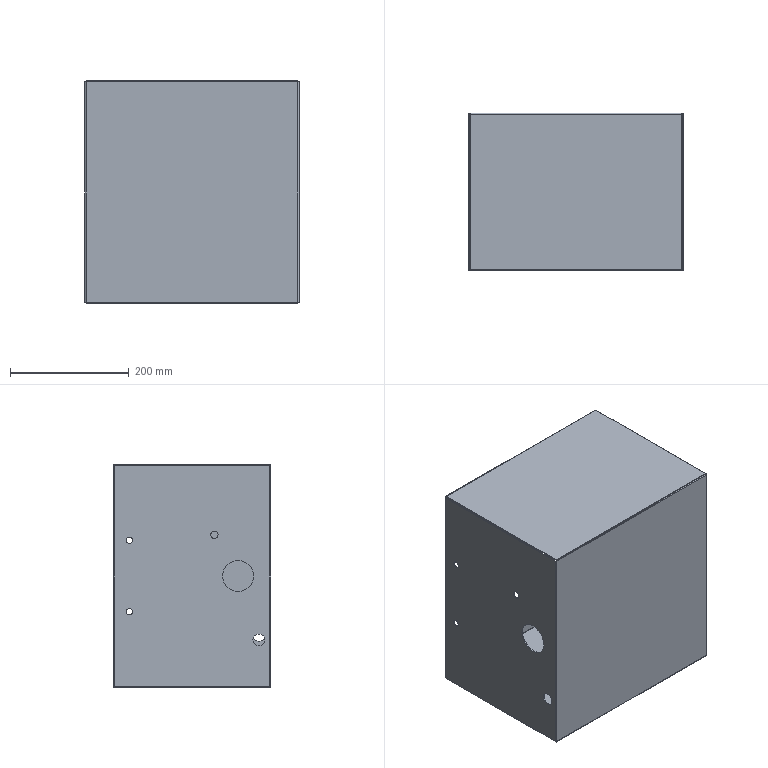Part | SolidWorks | features ICE 7, EdgeFlange 2, FlatPattern 1, SMBaseFlange 1, SheetMetal 1 | 1 solid | 94 faces | box 360 x 265 x 375 mm | volume 796453 mm3 | cylinder 40 | plane 38 | spline 16 | commonest cylinder face diameters 10.5 x12 1 x8 4 x8 20 x8 12.5 x2 52 x2